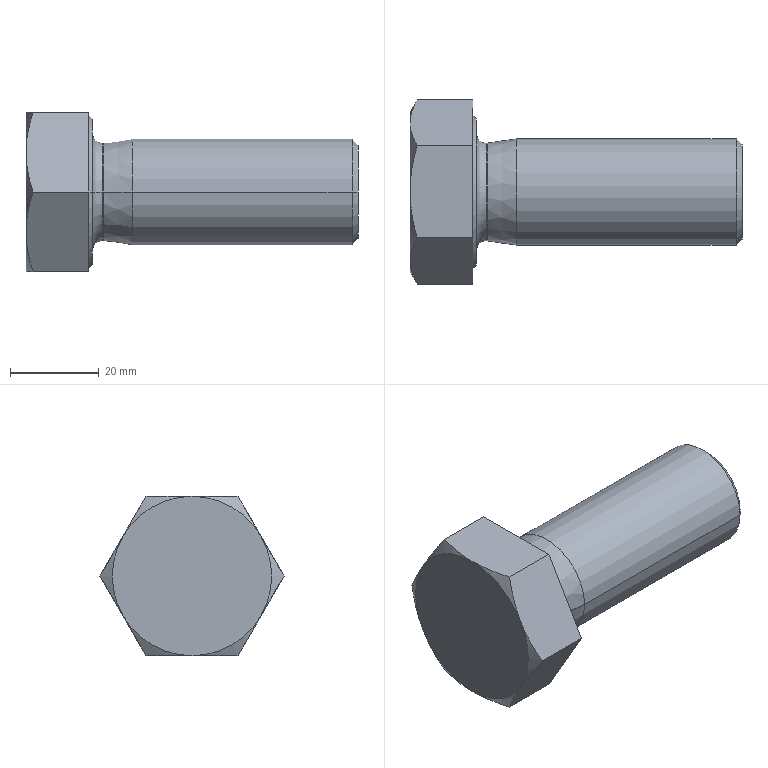Part | SolidWorks | features Chamfer 2, RevCut 2, Revolution 2, Extrusion 1, ICE 1 | 1 solid | 28 faces | box 75 x 41.569 x 36 mm | volume 43357 mm3 | cone 12 | plane 10 | torus 4 | cylinder 2 | commonest cylinder face diameters 24 x2
STEP:
#1=CARTESIAN_POINT('',(15.,-13.226,0.));
#2=VERTEX_POINT('',#1);
#3=CARTESIAN_POINT('',(17.2,-11.026,0.));
#4=VERTEX_POINT('',#3);
#5=CARTESIAN_POINT('',(17.2,-13.226,0.));
#6=DIRECTION('',(0.,0.,-1.));
#7=DIRECTION('',(-1.,0.,0.));
#8=AXIS2_PLACEMENT_3D('',#5,#6,#7);
#9=CIRCLE('',#8,2.2);
#10=EDGE_CURVE('',#2,#4,#9,.T.);
#11=ORIENTED_EDGE('',*,*,#10,.T.);
#12=CARTESIAN_POINT('',(17.2,11.026,0.));
#13=VERTEX_POINT('',#12);
#14=CARTESIAN_POINT('',(17.2,0.,0.));
#15=DIRECTION('',(-1.,0.,0.));
#16=DIRECTION('',(0.,-1.,0.));
#17=AXIS2_PLACEMENT_3D('',#14,#15,#16);
#18=CIRCLE('',#17,11.026);
#19=EDGE_CURVE('',#4,#13,#18,.T.);
#20=ORIENTED_EDGE('',*,*,#19,.T.);
#21=CARTESIAN_POINT('',(15.,13.226,0.));
#22=VERTEX_POINT('',#21);
#23=CARTESIAN_POINT('',(17.2,13.226,0.));
#24=DIRECTION('',(0.,0.,1.));
#25=DIRECTION('',(0.,-1.,0.));
#26=AXIS2_PLACEMENT_3D('',#23,#24,#25);
#27=CIRCLE('',#26,2.2);
#28=EDGE_CURVE('',#22,#13,#27,.T.);
#29=ORIENTED_EDGE('',*,*,#28,.F.);
#30=CARTESIAN_POINT('',(15.,0.,0.));
#31=DIRECTION('',(-1.,0.,0.));
#32=DIRECTION('',(0.,-1.,0.));
#33=AXIS2_PLACEMENT_3D('',#30,#31,#32);
#34=CIRCLE('',#33,13.226);
#35=EDGE_CURVE('',#2,#22,#34,.T.);
#36=ORIENTED_EDGE('',*,*,#35,.F.);
#37=EDGE_LOOP('',(#11,#20,#29,#36));
#38=FACE_OUTER_BOUND('',#37,.T.);
#39=CARTESIAN_POINT('',(17.2,0.,0.));
#40=DIRECTION('',(-1.,0.,0.));
#41=DIRECTION('',(0.,-1.,0.));
#42=AXIS2_PLACEMENT_3D('',#39,#40,#41);
#43=TOROIDAL_SURFACE('',#42,13.226,2.2);
#44=ADVANCED_FACE('',(#38),#43,.F.);
#45=ORIENTED_EDGE('',*,*,#28,.T.);
#46=CARTESIAN_POINT('',(17.2,0.,0.));
#47=DIRECTION('',(-1.,0.,0.));
#48=DIRECTION('',(0.,-1.,0.));
#49=AXIS2_PLACEMENT_3D('',#46,#47,#48);
#50=CIRCLE('',#49,11.026);
#51=EDGE_CURVE('',#13,#4,#50,.T.);
#52=ORIENTED_EDGE('',*,*,#51,.T.);
#53=ORIENTED_EDGE('',*,*,#10,.F.);
#54=CARTESIAN_POINT('',(15.,0.,0.));
#55=DIRECTION('',(-1.,0.,0.));
#56=DIRECTION('',(0.,-1.,0.));
#57=AXIS2_PLACEMENT_3D('',#54,#55,#56);
#58=CIRCLE('',#57,13.226);
#59=EDGE_CURVE('',#22,#2,#58,.T.);
#60=ORIENTED_EDGE('',*,*,#59,.F.);
#61=EDGE_LOOP('',(#45,#52,#53,#60));
#62=FACE_OUTER_BOUND('',#61,.T.);
#63=CARTESIAN_POINT('',(17.2,0.,0.));
#64=DIRECTION('',(-1.,0.,0.));
#65=DIRECTION('',(0.,-1.,0.));
#66=AXIS2_PLACEMENT_3D('',#63,#64,#65);
#67=TOROIDAL_SURFACE('',#66,13.226,2.2);
#68=ADVANCED_FACE('',(#62),#67,.F.);
#69=CARTESIAN_POINT('',(15.,-16.525,0.));
#70=VERTEX_POINT('',#69);
#71=CARTESIAN_POINT('',(15.,16.525,0.));
#72=VERTEX_POINT('',#71);
#73=CARTESIAN_POINT('',(15.,0.,0.));
#74=DIRECTION('',(-1.,0.,0.));
#75=DIRECTION('',(0.,-1.,0.));
#76=AXIS2_PLACEMENT_3D('',#73,#74,#75);
#77=CIRCLE('',#76,16.525);
#78=EDGE_CURVE('',#70,#72,#77,.T.);
#79=ORIENTED_EDGE('',*,*,#78,.T.);
#80=CARTESIAN_POINT('',(14.2,17.325,0.));
#81=VERTEX_POINT('',#80);
#82=CARTESIAN_POINT('',(14.2,17.325,0.));
#83=DIRECTION('',(-0.7071,0.7071,0.));
#84=VECTOR('',#83,1000.);
#85=LINE('',#82,#84);
#86=EDGE_CURVE('',#72,#81,#85,.T.);
#87=ORIENTED_EDGE('',*,*,#86,.T.);
#88=CARTESIAN_POINT('',(14.2,-17.325,0.));
#89=VERTEX_POINT('',#88);
#90=CARTESIAN_POINT('',(14.2,0.,0.));
#91=DIRECTION('',(-1.,0.,0.));
#92=DIRECTION('',(0.,-1.,0.));
#93=AXIS2_PLACEMENT_3D('',#90,#91,#92);
#94=CIRCLE('',#93,17.325);
#95=EDGE_CURVE('',#89,#81,#94,.T.);
#96=ORIENTED_EDGE('',*,*,#95,.F.);
#97=CARTESIAN_POINT('',(14.2,-17.325,0.));
#98=DIRECTION('',(-0.7071,-0.7071,0.));
#99=VECTOR('',#98,1000.);
#100=LINE('',#97,#99);
#101=EDGE_CURVE('',#70,#89,#100,.T.);
#102=ORIENTED_EDGE('',*,*,#101,.F.);
#103=EDGE_LOOP('',(#79,#87,#96,#102));
#104=FACE_OUTER_BOUND('',#103,.T.);
#105=CARTESIAN_POINT('',(14.2,0.,0.));
#106=DIRECTION('',(-1.,0.,0.));
#107=DIRECTION('',(0.,-1.,0.));
#108=AXIS2_PLACEMENT_3D('',#105,#106,#107);
#109=CONICAL_SURFACE('',#108,17.325,0.7854);
#110=ADVANCED_FACE('',(#104),#109,.T.);
#111=CARTESIAN_POINT('',(75.,10.667,0.));
#112=VERTEX_POINT('',#111);
#113=CARTESIAN_POINT('',(75.,-10.667,0.));
#114=VERTEX_POINT('',#113);
#115=CARTESIAN_POINT('',(75.,0.,0.));
#116=DIRECTION('',(1.,0.,0.));
#117=DIRECTION('',(0.,-1.,0.));
#118=AXIS2_PLACEMENT_3D('',#115,#116,#117);
#119=CIRCLE('',#118,10.667);
#120=EDGE_CURVE('',#112,#114,#119,.T.);
#121=ORIENTED_EDGE('',*,*,#120,.F.);
#122=CARTESIAN_POINT('',(73.667,12.,0.));
#123=VERTEX_POINT('',#122);
#124=CARTESIAN_POINT('',(73.667,12.,0.));
#125=DIRECTION('',(-0.7071,0.7071,0.));
#126=VECTOR('',#125,1000.);
#127=LINE('',#124,#126);
#128=EDGE_CURVE('',#112,#123,#127,.T.);
#129=ORIENTED_EDGE('',*,*,#128,.T.);
#130=CARTESIAN_POINT('',(73.667,-12.,0.));
#131=VERTEX_POINT('',#130);
#132=CARTESIAN_POINT('',(73.667,0.,0.));
#133=DIRECTION('',(-1.,0.,0.));
#134=DIRECTION('',(0.,-1.,0.));
#135=AXIS2_PLACEMENT_3D('',#132,#133,#134);
#136=CIRCLE('',#135,12.);
#137=EDGE_CURVE('',#131,#123,#136,.T.);
#138=ORIENTED_EDGE('',*,*,#137,.F.);
#139=CARTESIAN_POINT('',(73.667,-12.,0.));
#140=DIRECTION('',(-0.7071,-0.7071,0.));
#141=VECTOR('',#140,1000.);
#142=LINE('',#139,#141);
#143=EDGE_CURVE('',#114,#131,#142,.T.);
#144=ORIENTED_EDGE('',*,*,#143,.F.);
#145=EDGE_LOOP('',(#121,#129,#138,#144));
#146=FACE_OUTER_BOUND('',#145,.T.);
#147=CARTESIAN_POINT('',(73.667,0.,0.));
#148=DIRECTION('',(-1.,0.,0.));
#149=DIRECTION('',(0.,-1.,0.));
#150=AXIS2_PLACEMENT_3D('',#147,#148,#149);
#151=CONICAL_SURFACE('',#150,12.,0.7854);
#152=ADVANCED_FACE('',(#146),#151,.T.);
#153=ORIENTED_EDGE('',*,*,#51,.F.);
#154=CARTESIAN_POINT('',(17.519,11.049,0.));
#155=VERTEX_POINT('',#154);
#156=CARTESIAN_POINT('',(17.2,13.226,0.));
#157=DIRECTION('',(0.,0.,1.));
#158=DIRECTION('',(0.,-1.,0.));
#159=AXIS2_PLACEMENT_3D('',#156,#157,#158);
#160=CIRCLE('',#159,2.2);
#161=EDGE_CURVE('',#13,#155,#160,.T.);
#162=ORIENTED_EDGE('',*,*,#161,.T.);
#163=CARTESIAN_POINT('',(17.519,-11.049,0.));
#164=VERTEX_POINT('',#163);
#165=CARTESIAN_POINT('',(17.519,0.,0.));
#166=DIRECTION('',(-1.,0.,0.));
#167=DIRECTION('',(0.,-1.,0.));
#168=AXIS2_PLACEMENT_3D('',#165,#166,#167);
#169=CIRCLE('',#168,11.049);
#170=EDGE_CURVE('',#155,#164,#169,.T.);
#171=ORIENTED_EDGE('',*,*,#170,.T.);
#172=CARTESIAN_POINT('',(17.2,-13.226,0.));
#173=DIRECTION('',(0.,0.,-1.));
#174=DIRECTION('',(-1.,0.,0.));
#175=AXIS2_PLACEMENT_3D('',#172,#173,#174);
#176=CIRCLE('',#175,2.2);
#177=EDGE_CURVE('',#4,#164,#176,.T.);
#178=ORIENTED_EDGE('',*,*,#177,.F.);
#179=EDGE_LOOP('',(#153,#162,#171,#178));
#180=FACE_OUTER_BOUND('',#179,.T.);
#181=CARTESIAN_POINT('',(17.2,0.,0.));
#182=DIRECTION('',(-1.,0.,0.));
#183=DIRECTION('',(0.,-1.,0.));
#184=AXIS2_PLACEMENT_3D('',#181,#182,#183);
#185=TOROIDAL_SURFACE('',#184,13.226,2.2);
#186=ADVANCED_FACE('',(#180),#185,.F.);
#187=ORIENTED_EDGE('',*,*,#137,.T.);
#188=CARTESIAN_POINT('',(24.,12.,0.));
#189=VERTEX_POINT('',#188);
#190=CARTESIAN_POINT('',(15.,12.,0.));
#191=DIRECTION('',(-1.,0.,0.));
#192=VECTOR('',#191,1000.);
#193=LINE('',#190,#192);
#194=EDGE_CURVE('',#123,#189,#193,.T.);
#195=ORIENTED_EDGE('',*,*,#194,.T.);
#196=CARTESIAN_POINT('',(24.,-12.,0.));
#197=VERTEX_POINT('',#196);
#198=CARTESIAN_POINT('',(24.,0.,0.));
#199=DIRECTION('',(-1.,0.,0.));
#200=DIRECTION('',(0.,-1.,0.));
#201=AXIS2_PLACEMENT_3D('',#198,#199,#200);
#202=CIRCLE('',#201,12.);
#203=EDGE_CURVE('',#197,#189,#202,.T.);
#204=ORIENTED_EDGE('',*,*,#203,.F.);
#205=CARTESIAN_POINT('',(15.,-12.,0.));
#206=DIRECTION('',(-1.,0.,0.));
#207=VECTOR('',#206,1000.);
#208=LINE('',#205,#207);
#209=EDGE_CURVE('',#131,#197,#208,.T.);
#210=ORIENTED_EDGE('',*,*,#209,.F.);
#211=EDGE_LOOP('',(#187,#195,#204,#210));
#212=FACE_OUTER_BOUND('',#211,.T.);
#213=CARTESIAN_POINT('',(15.,0.,0.));
#214=DIRECTION('',(-1.,0.,0.));
#215=DIRECTION('',(0.,-1.,0.));
#216=AXIS2_PLACEMENT_3D('',#213,#214,#215);
#217=CYLINDRICAL_SURFACE('',#216,12.);
#218=ADVANCED_FACE('',(#212),#217,.T.);
#219=CARTESIAN_POINT('',(17.519,0.,0.));
#220=DIRECTION('',(-1.,0.,0.));
#221=DIRECTION('',(0.,-1.,0.));
#222=AXIS2_PLACEMENT_3D('',#219,#220,#221);
#223=CIRCLE('',#222,11.049);
#224=EDGE_CURVE('',#164,#155,#223,.T.);
#225=ORIENTED_EDGE('',*,*,#224,.F.);
#226=CARTESIAN_POINT('',(24.,-12.,0.));
#227=DIRECTION('',(0.9894,-0.1452,0.));
#228=VECTOR('',#227,1000.);
#229=LINE('',#226,#228);
#230=EDGE_CURVE('',#164,#197,#229,.T.);
#231=ORIENTED_EDGE('',*,*,#230,.T.);
#232=ORIENTED_EDGE('',*,*,#203,.T.);
#233=CARTESIAN_POINT('',(24.,12.,0.));
#234=DIRECTION('',(0.9894,0.1452,0.));
#235=VECTOR('',#234,1000.);
#236=LINE('',#233,#235);
#237=EDGE_CURVE('',#155,#189,#236,.T.);
#238=ORIENTED_EDGE('',*,*,#237,.F.);
#239=EDGE_LOOP('',(#225,#231,#232,#238));
#240=FACE_OUTER_BOUND('',#239,.T.);
#241=CARTESIAN_POINT('',(24.,0.,0.));
#242=DIRECTION('',(1.,0.,0.));
#243=DIRECTION('',(0.,1.,0.));
#244=AXIS2_PLACEMENT_3D('',#241,#242,#243);
#245=CONICAL_SURFACE('',#244,12.,0.1457);
#246=ADVANCED_FACE('',(#240),#245,.T.);
#247=ORIENTED_EDGE('',*,*,#35,.T.);
#248=ORIENTED_EDGE('',*,*,#59,.T.);
#249=EDGE_LOOP('',(#247,#248));
#250=FACE_BOUND('',#249,.T.);
#251=ORIENTED_EDGE('',*,*,#78,.F.);
#252=CARTESIAN_POINT('',(15.,0.,0.));
#253=DIRECTION('',(-1.,0.,0.));
#254=DIRECTION('',(0.,-1.,0.));
#255=AXIS2_PLACEMENT_3D('',#252,#253,#254);
#256=CIRCLE('',#255,16.525);
#257=EDGE_CURVE('',#72,#70,#256,.T.);
#258=ORIENTED_EDGE('',*,*,#257,.F.);
#259=EDGE_LOOP('',(#251,#258));
#260=FACE_OUTER_BOUND('',#259,.T.);
#261=CARTESIAN_POINT('',(15.,10.392,-18.));
#262=DIRECTION('',(1.,0.,0.));
#263=DIRECTION('',(0.,0.,-1.));
#264=AXIS2_PLACEMENT_3D('',#261,#262,#263);
#265=PLANE('',#264);
#266=ADVANCED_FACE('',(#250,#260),#265,.T.);
#267=ORIENTED_EDGE('',*,*,#230,.F.);
#268=ORIENTED_EDGE('',*,*,#170,.F.);
#269=ORIENTED_EDGE('',*,*,#237,.T.);
#270=CARTESIAN_POINT('',(24.,0.,0.));
#271=DIRECTION('',(-1.,0.,0.));
#272=DIRECTION('',(0.,-1.,0.));
#273=AXIS2_PLACEMENT_3D('',#270,#271,#272);
#274=CIRCLE('',#273,12.);
#275=EDGE_CURVE('',#189,#197,#274,.T.);
#276=ORIENTED_EDGE('',*,*,#275,.T.);
#277=EDGE_LOOP('',(#267,#268,#269,#276));
#278=FACE_OUTER_BOUND('',#277,.T.);
#279=CARTESIAN_POINT('',(24.,0.,0.));
#280=DIRECTION('',(1.,0.,0.));
#281=DIRECTION('',(0.,1.,0.));
#282=AXIS2_PLACEMENT_3D('',#279,#280,#281);
#283=CONICAL_SURFACE('',#282,12.,0.1457);
#284=ADVANCED_FACE('',(#278),#283,.T.);
#285=ORIENTED_EDGE('',*,*,#194,.F.);
#286=CARTESIAN_POINT('',(73.667,0.,0.));
#287=DIRECTION('',(-1.,0.,0.));
#288=DIRECTION('',(0.,-1.,0.));
#289=AXIS2_PLACEMENT_3D('',#286,#287,#288);
#290=CIRCLE('',#289,12.);
#291=EDGE_CURVE('',#123,#131,#290,.T.);
#292=ORIENTED_EDGE('',*,*,#291,.T.);
#293=ORIENTED_EDGE('',*,*,#209,.T.);
#294=ORIENTED_EDGE('',*,*,#275,.F.);
#295=EDGE_LOOP('',(#285,#292,#293,#294));
#296=FACE_OUTER_BOUND('',#295,.T.);
#297=CARTESIAN_POINT('',(15.,0.,0.));
#298=DIRECTION('',(-1.,0.,0.));
#299=DIRECTION('',(0.,-1.,0.));
#300=AXIS2_PLACEMENT_3D('',#297,#298,#299);
#301=CYLINDRICAL_SURFACE('',#300,12.);
#302=ADVANCED_FACE('',(#296),#301,.T.);
#303=CARTESIAN_POINT('',(75.,0.,0.));
#304=DIRECTION('',(1.,0.,0.));
#305=DIRECTION('',(0.,-1.,0.));
#306=AXIS2_PLACEMENT_3D('',#303,#304,#305);
#307=CIRCLE('',#306,10.667);
#308=EDGE_CURVE('',#114,#112,#307,.T.);
#309=ORIENTED_EDGE('',*,*,#308,.T.);
#310=ORIENTED_EDGE('',*,*,#120,.T.);
#311=EDGE_LOOP('',(#309,#310));
#312=FACE_OUTER_BOUND('',#311,.T.);
#313=CARTESIAN_POINT('',(75.,12.,0.));
#314=DIRECTION('',(-1.,0.,0.));
#315=DIRECTION('',(0.,-1.,0.));
#316=AXIS2_PLACEMENT_3D('',#313,#314,#315);
#317=PLANE('',#316);
#318=ADVANCED_FACE('',(#312),#317,.F.);
#319=ORIENTED_EDGE('',*,*,#19,.F.);
#320=ORIENTED_EDGE('',*,*,#177,.T.);
#321=ORIENTED_EDGE('',*,*,#224,.T.);
#322=ORIENTED_EDGE('',*,*,#161,.F.);
#323=EDGE_LOOP('',(#319,#320,#321,#322));
#324=FACE_OUTER_BOUND('',#323,.T.);
#325=CARTESIAN_POINT('',(17.2,0.,0.));
#326=DIRECTION('',(-1.,0.,0.));
#327=DIRECTION('',(0.,-1.,0.));
#328=AXIS2_PLACEMENT_3D('',#325,#326,#327);
#329=TOROIDAL_SURFACE('',#328,13.226,2.2);
#330=ADVANCED_FACE('',(#324),#329,.F.);
#331=ORIENTED_EDGE('',*,*,#128,.F.);
#332=ORIENTED_EDGE('',*,*,#308,.F.);
#333=ORIENTED_EDGE('',*,*,#143,.T.);
#334=ORIENTED_EDGE('',*,*,#291,.F.);
#335=EDGE_LOOP('',(#331,#332,#333,#334));
#336=FACE_OUTER_BOUND('',#335,.T.);
#337=CARTESIAN_POINT('',(73.667,0.,0.));
#338=DIRECTION('',(-1.,0.,0.));
#339=DIRECTION('',(0.,-1.,0.));
#340=AXIS2_PLACEMENT_3D('',#337,#338,#339);
#341=CONICAL_SURFACE('',#340,12.,0.7854);
#342=ADVANCED_FACE('',(#336),#341,.T.);
#343=ORIENTED_EDGE('',*,*,#95,.T.);
#344=CARTESIAN_POINT('',(14.2,0.,0.));
#345=DIRECTION('',(-1.,0.,0.));
#346=DIRECTION('',(0.,-1.,0.));
#347=AXIS2_PLACEMENT_3D('',#344,#345,#346);
#348=CIRCLE('',#347,17.325);
#349=EDGE_CURVE('',#81,#89,#348,.T.);
#350=ORIENTED_EDGE('',*,*,#349,.T.);
#351=EDGE_LOOP('',(#343,#350));
#352=FACE_BOUND('',#351,.T.);
#353=CARTESIAN_POINT('',(14.2,-10.392,-18.));
#354=VERTEX_POINT('',#353);
#355=CARTESIAN_POINT('',(14.2,10.392,-18.));
#356=VERTEX_POINT('',#355);
#357=CARTESIAN_POINT('',(14.2,-10.392,-18.));
#358=DIRECTION('',(0.,1.,0.));
#359=VECTOR('',#358,1000.);
#360=LINE('',#357,#359);
#361=EDGE_CURVE('',#354,#356,#360,.T.);
#362=ORIENTED_EDGE('',*,*,#361,.T.);
#363=CARTESIAN_POINT('',(14.2,20.785,0.));
#364=VERTEX_POINT('',#363);
#365=CARTESIAN_POINT('',(14.2,10.392,-18.));
#366=DIRECTION('',(0.,0.5,0.866));
#367=VECTOR('',#366,1000.);
#368=LINE('',#365,#367);
#369=EDGE_CURVE('',#356,#364,#368,.T.);
#370=ORIENTED_EDGE('',*,*,#369,.T.);
#371=CARTESIAN_POINT('',(14.2,10.392,18.));
#372=VERTEX_POINT('',#371);
#373=CARTESIAN_POINT('',(14.2,20.785,0.));
#374=DIRECTION('',(0.,-0.5,0.866));
#375=VECTOR('',#374,1000.);
#376=LINE('',#373,#375);
#377=EDGE_CURVE('',#364,#372,#376,.T.);
#378=ORIENTED_EDGE('',*,*,#377,.T.);
#379=CARTESIAN_POINT('',(14.2,-10.392,18.));
#380=VERTEX_POINT('',#379);
#381=CARTESIAN_POINT('',(14.2,10.392,18.));
#382=DIRECTION('',(0.,-1.,0.));
#383=VECTOR('',#382,1000.);
#384=LINE('',#381,#383);
#385=EDGE_CURVE('',#372,#380,#384,.T.);
#386=ORIENTED_EDGE('',*,*,#385,.T.);
#387=CARTESIAN_POINT('',(14.2,-20.785,0.));
#388=VERTEX_POINT('',#387);
#389=CARTESIAN_POINT('',(14.2,-10.392,18.));
#390=DIRECTION('',(0.,-0.5,-0.866));
#391=VECTOR('',#390,1000.);
#392=LINE('',#389,#391);
#393=EDGE_CURVE('',#380,#388,#392,.T.);
#394=ORIENTED_EDGE('',*,*,#393,.T.);
#395=CARTESIAN_POINT('',(14.2,-20.785,0.));
#396=DIRECTION('',(0.,0.5,-0.866));
#397=VECTOR('',#396,1000.);
#398=LINE('',#395,#397);
#399=EDGE_CURVE('',#388,#354,#398,.T.);
#400=ORIENTED_EDGE('',*,*,#399,.T.);
#401=EDGE_LOOP('',(#362,#370,#378,#386,#394,#400));
#402=FACE_OUTER_BOUND('',#401,.T.);
#403=CARTESIAN_POINT('',(14.2,-17.325,0.));
#404=DIRECTION('',(1.,0.,0.));
#405=DIRECTION('',(0.,1.,0.));
#406=AXIS2_PLACEMENT_3D('',#403,#404,#405);
#407=PLANE('',#406);
#408=ADVANCED_FACE('',(#352,#402),#407,.T.);
#409=ORIENTED_EDGE('',*,*,#86,.F.);
#410=ORIENTED_EDGE('',*,*,#257,.T.);
#411=ORIENTED_EDGE('',*,*,#101,.T.);
#412=ORIENTED_EDGE('',*,*,#349,.F.);
#413=EDGE_LOOP('',(#409,#410,#411,#412));
#414=FACE_OUTER_BOUND('',#413,.T.);
#415=CARTESIAN_POINT('',(14.2,0.,0.));
#416=DIRECTION('',(-1.,0.,0.));
#417=DIRECTION('',(0.,-1.,0.));
#418=AXIS2_PLACEMENT_3D('',#415,#416,#417);
#419=CONICAL_SURFACE('',#418,17.325,0.7854);
#420=ADVANCED_FACE('',(#414),#419,.T.);
#421=CARTESIAN_POINT('',(0.,0.,-18.));
#422=VERTEX_POINT('',#421);
#423=CARTESIAN_POINT('',(0.,15.588,-9.));
#424=VERTEX_POINT('',#423);
#425=CARTESIAN_POINT('',(0.,0.,0.));
#426=DIRECTION('',(1.,0.,0.));
#427=DIRECTION('',(0.,0.,-1.));
#428=AXIS2_PLACEMENT_3D('',#425,#426,#427);
#429=CIRCLE('',#428,18.);
#430=EDGE_CURVE('',#422,#424,#429,.T.);
#431=ORIENTED_EDGE('',*,*,#430,.F.);
#432=CARTESIAN_POINT('',(0.,-15.588,-9.));
#433=VERTEX_POINT('',#432);
#434=CARTESIAN_POINT('',(0.,0.,0.));
#435=DIRECTION('',(1.,0.,0.));
#436=DIRECTION('',(0.,0.,-1.));
#437=AXIS2_PLACEMENT_3D('',#434,#435,#436);
#438=CIRCLE('',#437,18.);
#439=EDGE_CURVE('',#433,#422,#438,.T.);
#440=ORIENTED_EDGE('',*,*,#439,.F.);
#441=CARTESIAN_POINT('',(0.,-15.588,9.));
#442=VERTEX_POINT('',#441);
#443=CARTESIAN_POINT('',(0.,0.,0.));
#444=DIRECTION('',(1.,0.,0.));
#445=DIRECTION('',(0.,0.,-1.));
#446=AXIS2_PLACEMENT_3D('',#443,#444,#445);
#447=CIRCLE('',#446,18.);
#448=EDGE_CURVE('',#442,#433,#447,.T.);
#449=ORIENTED_EDGE('',*,*,#448,.F.);
#450=CARTESIAN_POINT('',(0.,0.,18.));
#451=VERTEX_POINT('',#450);
#452=CARTESIAN_POINT('',(0.,0.,0.));
#453=DIRECTION('',(1.,0.,0.));
#454=DIRECTION('',(0.,0.,-1.));
#455=AXIS2_PLACEMENT_3D('',#452,#453,#454);
#456=CIRCLE('',#455,18.);
#457=EDGE_CURVE('',#451,#442,#456,.T.);
#458=ORIENTED_EDGE('',*,*,#457,.F.);
#459=CARTESIAN_POINT('',(0.,15.588,9.));
#460=VERTEX_POINT('',#459);
#461=CARTESIAN_POINT('',(0.,0.,0.));
#462=DIRECTION('',(-1.,0.,0.));
#463=DIRECTION('',(0.,0.,1.));
#464=AXIS2_PLACEMENT_3D('',#461,#462,#463);
#465=CIRCLE('',#464,18.);
#466=EDGE_CURVE('',#451,#460,#465,.T.);
#467=ORIENTED_EDGE('',*,*,#466,.T.);
#468=CARTESIAN_POINT('',(0.,0.,0.));
#469=DIRECTION('',(1.,0.,0.));
#470=DIRECTION('',(0.,0.,-1.));
#471=AXIS2_PLACEMENT_3D('',#468,#469,#470);
#472=CIRCLE('',#471,18.);
#473=EDGE_CURVE('',#424,#460,#472,.T.);
#474=ORIENTED_EDGE('',*,*,#473,.F.);
#475=EDGE_LOOP('',(#431,#440,#449,#458,#467,#474));
#476=FACE_OUTER_BOUND('',#475,.T.);
#477=CARTESIAN_POINT('',(0.,10.392,-18.));
#478=DIRECTION('',(1.,0.,0.));
#479=DIRECTION('',(0.,0.,-1.));
#480=AXIS2_PLACEMENT_3D('',#477,#478,#479);
#481=PLANE('',#480);
#482=ADVANCED_FACE('',(#476),#481,.F.);
#483=CARTESIAN_POINT('',(1.608,10.392,-18.));
#484=VERTEX_POINT('',#483);
#485=CARTESIAN_POINT('',(0.,15.588,-9.));
#486=CARTESIAN_POINT('',(0.,15.368,-9.382));
#487=CARTESIAN_POINT('',(0.009429,15.146,-9.766));
#488=CARTESIAN_POINT('',(0.04683,14.705,-10.53));
#489=CARTESIAN_POINT('',(0.07476,14.485,-10.91));
#490=CARTESIAN_POINT('',(0.1851,13.828,-12.049));
#491=CARTESIAN_POINT('',(0.294,13.393,-12.803));
#492=CARTESIAN_POINT('',(0.714,12.095,-15.051));
#493=CARTESIAN_POINT('',(1.118,11.24,-16.531));
#494=CARTESIAN_POINT('',(1.608,10.392,-18.));
#495=B_SPLINE_CURVE_WITH_KNOTS('',3,(#485,#486,#487,#488,#489,#490,#491,#492,#493,#494),.UNSPECIFIED.,.F.,.F.,(4,2,2,2,4),(0.01052,0.01183,0.01313,0.01575,0.02099),.UNSPECIFIED.);
#496=EDGE_CURVE('',#424,#484,#495,.T.);
#497=ORIENTED_EDGE('',*,*,#496,.T.);
#498=CARTESIAN_POINT('',(1.608,10.392,-18.));
#499=CARTESIAN_POINT('',(1.123,8.712,-18.));
#500=CARTESIAN_POINT('',(0.7186,7.01,-18.));
#501=CARTESIAN_POINT('',(0.296,4.406,-18.));
#502=CARTESIAN_POINT('',(0.1858,3.529,-18.));
#503=CARTESIAN_POINT('',(0.03734,1.76,-18.));
#504=CARTESIAN_POINT('',(0.,0.8787,-18.));
#505=CARTESIAN_POINT('',(0.,0.,-18.));
#506=B_SPLINE_CURVE_WITH_KNOTS('',3,(#498,#499,#500,#501,#502,#503,#504,#505),.UNSPECIFIED.,.F.,.F.,(4,2,2,4),(0.007574,0.01282,0.01544,0.01807),.UNSPECIFIED.);
#507=EDGE_CURVE('',#484,#422,#506,.T.);
#508=ORIENTED_EDGE('',*,*,#507,.T.);
#509=ORIENTED_EDGE('',*,*,#430,.T.);
#510=EDGE_LOOP('',(#497,#508,#509));
#511=FACE_OUTER_BOUND('',#510,.T.);
#512=CARTESIAN_POINT('',(0.,0.,0.));
#513=DIRECTION('',(1.,0.,0.));
#514=DIRECTION('',(0.,0.,1.));
#515=AXIS2_PLACEMENT_3D('',#512,#513,#514);
#516=CONICAL_SURFACE('',#515,18.,1.047);
#517=ADVANCED_FACE('',(#511),#516,.T.);
#518=CARTESIAN_POINT('',(1.608,20.785,0.));
#519=VERTEX_POINT('',#518);
#520=CARTESIAN_POINT('',(0.,15.588,9.));
#521=CARTESIAN_POINT('',(0.,15.809,8.618));
#522=CARTESIAN_POINT('',(0.009429,16.031,8.234));
#523=CARTESIAN_POINT('',(0.04683,16.472,7.47));
#524=CARTESIAN_POINT('',(0.07476,16.691,7.09));
#525=CARTESIAN_POINT('',(0.1851,17.349,5.951));
#526=CARTESIAN_POINT('',(0.294,17.784,5.197));
#527=CARTESIAN_POINT('',(0.714,19.082,2.949));
#528=CARTESIAN_POINT('',(1.118,19.937,1.469));
#529=CARTESIAN_POINT('',(1.608,20.785,0.));
#530=B_SPLINE_CURVE_WITH_KNOTS('',3,(#520,#521,#522,#523,#524,#525,#526,#527,#528,#529),.UNSPECIFIED.,.F.,.F.,(4,2,2,2,4),(0.01052,0.01183,0.01313,0.01575,0.02099),.UNSPECIFIED.);
#531=EDGE_CURVE('',#460,#519,#530,.T.);
#532=ORIENTED_EDGE('',*,*,#531,.T.);
#533=CARTESIAN_POINT('',(1.608,20.785,0.));
#534=CARTESIAN_POINT('',(1.117,19.935,-1.472));
#535=CARTESIAN_POINT('',(0.7126,19.078,-2.955));
#536=CARTESIAN_POINT('',(0.1532,17.348,-5.952));
#537=CARTESIAN_POINT('',(0.,16.474,-7.467));
#538=CARTESIAN_POINT('',(0.,15.588,-9.));
#539=B_SPLINE_CURVE_WITH_KNOTS('',3,(#533,#534,#535,#536,#537,#538),.UNSPECIFIED.,.F.,.F.,(4,2,4),(0.000000238,0.005258,0.01052),.UNSPECIFIED.);
#540=EDGE_CURVE('',#519,#424,#539,.T.);
#541=ORIENTED_EDGE('',*,*,#540,.T.);
#542=ORIENTED_EDGE('',*,*,#473,.T.);
#543=EDGE_LOOP('',(#532,#541,#542));
#544=FACE_OUTER_BOUND('',#543,.T.);
#545=CARTESIAN_POINT('',(0.,0.,0.));
#546=DIRECTION('',(1.,0.,0.));
#547=DIRECTION('',(0.,0.,1.));
#548=AXIS2_PLACEMENT_3D('',#545,#546,#547);
#549=CONICAL_SURFACE('',#548,18.,1.047);
#550=ADVANCED_FACE('',(#544),#549,.T.);
#551=CARTESIAN_POINT('',(1.608,10.392,18.));
#552=VERTEX_POINT('',#551);
#553=CARTESIAN_POINT('',(1.608,10.392,18.));
#554=CARTESIAN_POINT('',(1.117,11.242,16.528));
#555=CARTESIAN_POINT('',(0.7126,12.099,15.045));
#556=CARTESIAN_POINT('',(0.1532,13.829,12.048));
#557=CARTESIAN_POINT('',(0.,14.703,10.533));
#558=CARTESIAN_POINT('',(0.,15.588,9.));
#559=B_SPLINE_CURVE_WITH_KNOTS('',3,(#553,#554,#555,#556,#557,#558),.UNSPECIFIED.,.F.,.F.,(4,2,4),(0.000000238,0.005258,0.01052),.UNSPECIFIED.);
#560=EDGE_CURVE('',#552,#460,#559,.T.);
#561=ORIENTED_EDGE('',*,*,#560,.T.);
#562=ORIENTED_EDGE('',*,*,#466,.F.);
#563=CARTESIAN_POINT('',(0.,0.,18.));
#564=CARTESIAN_POINT('',(0.,0.8787,18.));
#565=CARTESIAN_POINT('',(0.03734,1.76,18.));
#566=CARTESIAN_POINT('',(0.1858,3.529,18.));
#567=CARTESIAN_POINT('',(0.296,4.406,18.));
#568=CARTESIAN_POINT('',(0.7186,7.01,18.));
#569=CARTESIAN_POINT('',(1.123,8.712,18.));
#570=CARTESIAN_POINT('',(1.608,10.392,18.));
#571=B_SPLINE_CURVE_WITH_KNOTS('',3,(#563,#564,#565,#566,#567,#568,#569,#570),.UNSPECIFIED.,.F.,.F.,(4,2,2,4),(0.0291,0.03173,0.03436,0.03962),.UNSPECIFIED.);
#572=EDGE_CURVE('',#451,#552,#571,.T.);
#573=ORIENTED_EDGE('',*,*,#572,.T.);
#574=EDGE_LOOP('',(#561,#562,#573));
#575=FACE_OUTER_BOUND('',#574,.T.);
#576=CARTESIAN_POINT('',(0.,0.,0.));
#577=DIRECTION('',(1.,0.,0.));
#578=DIRECTION('',(0.,0.,1.));
#579=AXIS2_PLACEMENT_3D('',#576,#577,#578);
#580=CONICAL_SURFACE('',#579,18.,1.047);
#581=ADVANCED_FACE('',(#575),#580,.T.);
#582=CARTESIAN_POINT('',(1.608,-10.392,18.));
#583=VERTEX_POINT('',#582);
#584=CARTESIAN_POINT('',(1.608,-10.392,18.));
#585=CARTESIAN_POINT('',(1.364,-9.547,18.));
#586=CARTESIAN_POINT('',(1.14,-8.694,18.));
#587=CARTESIAN_POINT('',(0.7423,-6.969,18.));
#588=CARTESIAN_POINT('',(0.5706,-6.103,18.));
#589=CARTESIAN_POINT('',(0.151,-3.501,18.));
#590=CARTESIAN_POINT('',(0.,-1.756,18.));
#591=CARTESIAN_POINT('',(0.,0.,18.));
#592=B_SPLINE_CURVE_WITH_KNOTS('',3,(#584,#585,#586,#587,#588,#589,#590,#591),.UNSPECIFIED.,.F.,.F.,(4,2,2,4),(0.01858,0.02121,0.02384,0.0291),.UNSPECIFIED.);
#593=EDGE_CURVE('',#583,#451,#592,.T.);
#594=ORIENTED_EDGE('',*,*,#593,.T.);
#595=ORIENTED_EDGE('',*,*,#457,.T.);
#596=CARTESIAN_POINT('',(0.,-15.588,9.));
#597=CARTESIAN_POINT('',(0.,-15.368,9.382));
#598=CARTESIAN_POINT('',(0.009429,-15.146,9.766));
#599=CARTESIAN_POINT('',(0.04683,-14.705,10.53));
#600=CARTESIAN_POINT('',(0.07476,-14.485,10.91));
#601=CARTESIAN_POINT('',(0.1851,-13.828,12.049));
#602=CARTESIAN_POINT('',(0.294,-13.393,12.803));
#603=CARTESIAN_POINT('',(0.714,-12.095,15.051));
#604=CARTESIAN_POINT('',(1.118,-11.24,16.531));
#605=CARTESIAN_POINT('',(1.608,-10.392,18.));
#606=B_SPLINE_CURVE_WITH_KNOTS('',3,(#596,#597,#598,#599,#600,#601,#602,#603,#604,#605),.UNSPECIFIED.,.F.,.F.,(4,2,2,2,4),(0.01052,0.01183,0.01313,0.01575,0.02099),.UNSPECIFIED.);
#607=EDGE_CURVE('',#442,#583,#606,.T.);
#608=ORIENTED_EDGE('',*,*,#607,.T.);
#609=EDGE_LOOP('',(#594,#595,#608));
#610=FACE_OUTER_BOUND('',#609,.T.);
#611=CARTESIAN_POINT('',(0.,0.,0.));
#612=DIRECTION('',(1.,0.,0.));
#613=DIRECTION('',(0.,0.,1.));
#614=AXIS2_PLACEMENT_3D('',#611,#612,#613);
#615=CONICAL_SURFACE('',#614,18.,1.047);
#616=ADVANCED_FACE('',(#610),#615,.T.);
#617=CARTESIAN_POINT('',(1.608,-10.392,-18.));
#618=VERTEX_POINT('',#617);
#619=CARTESIAN_POINT('',(0.,0.,-18.));
#620=CARTESIAN_POINT('',(0.,-1.756,-18.));
#621=CARTESIAN_POINT('',(0.151,-3.501,-18.));
#622=CARTESIAN_POINT('',(0.5706,-6.103,-18.));
#623=CARTESIAN_POINT('',(0.7423,-6.969,-18.));
#624=CARTESIAN_POINT('',(1.14,-8.694,-18.));
#625=CARTESIAN_POINT('',(1.364,-9.547,-18.));
#626=CARTESIAN_POINT('',(1.608,-10.392,-18.));
#627=B_SPLINE_CURVE_WITH_KNOTS('',3,(#619,#620,#621,#622,#623,#624,#625,#626),.UNSPECIFIED.,.F.,.F.,(4,2,2,4),(0.01807,0.02331,0.02593,0.02855),.UNSPECIFIED.);
#628=EDGE_CURVE('',#422,#618,#627,.T.);
#629=ORIENTED_EDGE('',*,*,#628,.T.);
#630=CARTESIAN_POINT('',(1.608,-10.392,-18.));
#631=CARTESIAN_POINT('',(1.117,-11.242,-16.528));
#632=CARTESIAN_POINT('',(0.7126,-12.099,-15.045));
#633=CARTESIAN_POINT('',(0.1532,-13.829,-12.048));
#634=CARTESIAN_POINT('',(0.,-14.703,-10.533));
#635=CARTESIAN_POINT('',(0.,-15.588,-9.));
#636=B_SPLINE_CURVE_WITH_KNOTS('',3,(#630,#631,#632,#633,#634,#635),.UNSPECIFIED.,.F.,.F.,(4,2,4),(0.000000238,0.005258,0.01052),.UNSPECIFIED.);
#637=EDGE_CURVE('',#618,#433,#636,.T.);
#638=ORIENTED_EDGE('',*,*,#637,.T.);
#639=ORIENTED_EDGE('',*,*,#439,.T.);
#640=EDGE_LOOP('',(#629,#638,#639));
#641=FACE_OUTER_BOUND('',#640,.T.);
#642=CARTESIAN_POINT('',(0.,0.,0.));
#643=DIRECTION('',(1.,0.,0.));
#644=DIRECTION('',(0.,0.,1.));
#645=AXIS2_PLACEMENT_3D('',#642,#643,#644);
#646=CONICAL_SURFACE('',#645,18.,1.047);
#647=ADVANCED_FACE('',(#641),#646,.T.);
#648=CARTESIAN_POINT('',(1.608,-20.785,0.));
#649=VERTEX_POINT('',#648);
#650=CARTESIAN_POINT('',(1.608,-20.785,0.));
#651=CARTESIAN_POINT('',(1.117,-19.935,1.472));
#652=CARTESIAN_POINT('',(0.7126,-19.078,2.955));
#653=CARTESIAN_POINT('',(0.1532,-17.348,5.952));
#654=CARTESIAN_POINT('',(0.,-16.474,7.467));
#655=CARTESIAN_POINT('',(0.,-15.588,9.));
#656=B_SPLINE_CURVE_WITH_KNOTS('',3,(#650,#651,#652,#653,#654,#655),.UNSPECIFIED.,.F.,.F.,(4,2,4),(0.000000238,0.005258,0.01052),.UNSPECIFIED.);
#657=EDGE_CURVE('',#649,#442,#656,.T.);
#658=ORIENTED_EDGE('',*,*,#657,.T.);
#659=ORIENTED_EDGE('',*,*,#448,.T.);
#660=CARTESIAN_POINT('',(0.,-15.588,-9.));
#661=CARTESIAN_POINT('',(0.,-15.809,-8.618));
#662=CARTESIAN_POINT('',(0.009429,-16.031,-8.234));
#663=CARTESIAN_POINT('',(0.04683,-16.472,-7.47));
#664=CARTESIAN_POINT('',(0.07476,-16.691,-7.09));
#665=CARTESIAN_POINT('',(0.1851,-17.349,-5.951));
#666=CARTESIAN_POINT('',(0.294,-17.784,-5.197));
#667=CARTESIAN_POINT('',(0.714,-19.082,-2.949));
#668=CARTESIAN_POINT('',(1.118,-19.937,-1.469));
#669=CARTESIAN_POINT('',(1.608,-20.785,0.));
#670=B_SPLINE_CURVE_WITH_KNOTS('',3,(#660,#661,#662,#663,#664,#665,#666,#667,#668,#669),.UNSPECIFIED.,.F.,.F.,(4,2,2,2,4),(0.01052,0.01183,0.01313,0.01575,0.02099),.UNSPECIFIED.);
#671=EDGE_CURVE('',#433,#649,#670,.T.);
#672=ORIENTED_EDGE('',*,*,#671,.T.);
#673=EDGE_LOOP('',(#658,#659,#672));
#674=FACE_OUTER_BOUND('',#673,.T.);
#675=CARTESIAN_POINT('',(0.,0.,0.));
#676=DIRECTION('',(1.,0.,0.));
#677=DIRECTION('',(0.,0.,1.));
#678=AXIS2_PLACEMENT_3D('',#675,#676,#677);
#679=CONICAL_SURFACE('',#678,18.,1.047);
#680=ADVANCED_FACE('',(#674),#679,.T.);
#681=ORIENTED_EDGE('',*,*,#399,.F.);
#682=CARTESIAN_POINT('',(15.,-20.785,0.));
#683=DIRECTION('',(-1.,0.,0.));
#684=VECTOR('',#683,1000.);
#685=LINE('',#682,#684);
#686=EDGE_CURVE('',#388,#649,#685,.T.);
#687=ORIENTED_EDGE('',*,*,#686,.T.);
#688=ORIENTED_EDGE('',*,*,#671,.F.);
#689=ORIENTED_EDGE('',*,*,#637,.F.);
#690=CARTESIAN_POINT('',(15.,-10.392,-18.));
#691=DIRECTION('',(-1.,0.,0.));
#692=VECTOR('',#691,1000.);
#693=LINE('',#690,#692);
#694=EDGE_CURVE('',#354,#618,#693,.T.);
#695=ORIENTED_EDGE('',*,*,#694,.F.);
#696=EDGE_LOOP('',(#681,#687,#688,#689,#695));
#697=FACE_OUTER_BOUND('',#696,.T.);
#698=CARTESIAN_POINT('',(15.,-20.785,0.));
#699=DIRECTION('',(0.,0.866,0.5));
#700=DIRECTION('',(0.,-0.5,0.866));
#701=AXIS2_PLACEMENT_3D('',#698,#699,#700);
#702=PLANE('',#701);
#703=ADVANCED_FACE('',(#697),#702,.F.);
#704=ORIENTED_EDGE('',*,*,#393,.F.);
#705=CARTESIAN_POINT('',(15.,-10.392,18.));
#706=DIRECTION('',(-1.,0.,0.));
#707=VECTOR('',#706,1000.);
#708=LINE('',#705,#707);
#709=EDGE_CURVE('',#380,#583,#708,.T.);
#710=ORIENTED_EDGE('',*,*,#709,.T.);
#711=ORIENTED_EDGE('',*,*,#607,.F.);
#712=ORIENTED_EDGE('',*,*,#657,.F.);
#713=ORIENTED_EDGE('',*,*,#686,.F.);
#714=EDGE_LOOP('',(#704,#710,#711,#712,#713));
#715=FACE_OUTER_BOUND('',#714,.T.);
#716=CARTESIAN_POINT('',(15.,-10.392,18.));
#717=DIRECTION('',(0.,0.866,-0.5));
#718=DIRECTION('',(0.,0.5,0.866));
#719=AXIS2_PLACEMENT_3D('',#716,#717,#718);
#720=PLANE('',#719);
#721=ADVANCED_FACE('',(#715),#720,.F.);
#722=ORIENTED_EDGE('',*,*,#385,.F.);
#723=CARTESIAN_POINT('',(15.,10.392,18.));
#724=DIRECTION('',(-1.,0.,0.));
#725=VECTOR('',#724,1000.);
#726=LINE('',#723,#725);
#727=EDGE_CURVE('',#372,#552,#726,.T.);
#728=ORIENTED_EDGE('',*,*,#727,.T.);
#729=ORIENTED_EDGE('',*,*,#572,.F.);
#730=ORIENTED_EDGE('',*,*,#593,.F.);
#731=ORIENTED_EDGE('',*,*,#709,.F.);
#732=EDGE_LOOP('',(#722,#728,#729,#730,#731));
#733=FACE_OUTER_BOUND('',#732,.T.);
#734=CARTESIAN_POINT('',(15.,10.392,18.));
#735=DIRECTION('',(0.,0.,-1.));
#736=DIRECTION('',(0.,1.,0.));
#737=AXIS2_PLACEMENT_3D('',#734,#735,#736);
#738=PLANE('',#737);
#739=ADVANCED_FACE('',(#733),#738,.F.);
#740=ORIENTED_EDGE('',*,*,#377,.F.);
#741=CARTESIAN_POINT('',(15.,20.785,0.));
#742=DIRECTION('',(-1.,0.,0.));
#743=VECTOR('',#742,1000.);
#744=LINE('',#741,#743);
#745=EDGE_CURVE('',#364,#519,#744,.T.);
#746=ORIENTED_EDGE('',*,*,#745,.T.);
#747=ORIENTED_EDGE('',*,*,#531,.F.);
#748=ORIENTED_EDGE('',*,*,#560,.F.);
#749=ORIENTED_EDGE('',*,*,#727,.F.);
#750=EDGE_LOOP('',(#740,#746,#747,#748,#749));
#751=FACE_OUTER_BOUND('',#750,.T.);
#752=CARTESIAN_POINT('',(15.,20.785,0.));
#753=DIRECTION('',(0.,-0.866,-0.5));
#754=DIRECTION('',(0.,0.5,-0.866));
#755=AXIS2_PLACEMENT_3D('',#752,#753,#754);
#756=PLANE('',#755);
#757=ADVANCED_FACE('',(#751),#756,.F.);
#758=ORIENTED_EDGE('',*,*,#369,.F.);
#759=CARTESIAN_POINT('',(15.,10.392,-18.));
#760=DIRECTION('',(-1.,0.,0.));
#761=VECTOR('',#760,1000.);
#762=LINE('',#759,#761);
#763=EDGE_CURVE('',#356,#484,#762,.T.);
#764=ORIENTED_EDGE('',*,*,#763,.T.);
#765=ORIENTED_EDGE('',*,*,#496,.F.);
#766=ORIENTED_EDGE('',*,*,#540,.F.);
#767=ORIENTED_EDGE('',*,*,#745,.F.);
#768=EDGE_LOOP('',(#758,#764,#765,#766,#767));
#769=FACE_OUTER_BOUND('',#768,.T.);
#770=CARTESIAN_POINT('',(15.,10.392,-18.));
#771=DIRECTION('',(0.,-0.866,0.5));
#772=DIRECTION('',(0.,-0.5,-0.866));
#773=AXIS2_PLACEMENT_3D('',#770,#771,#772);
#774=PLANE('',#773);
#775=ADVANCED_FACE('',(#769),#774,.F.);
#776=ORIENTED_EDGE('',*,*,#361,.F.);
#777=ORIENTED_EDGE('',*,*,#694,.T.);
#778=ORIENTED_EDGE('',*,*,#628,.F.);
#779=ORIENTED_EDGE('',*,*,#507,.F.);
#780=ORIENTED_EDGE('',*,*,#763,.F.);
#781=EDGE_LOOP('',(#776,#777,#778,#779,#780));
#782=FACE_OUTER_BOUND('',#781,.T.);
#783=CARTESIAN_POINT('',(15.,-10.392,-18.));
#784=DIRECTION('',(0.,0.,1.));
#785=DIRECTION('',(0.,-1.,0.));
#786=AXIS2_PLACEMENT_3D('',#783,#784,#785);
#787=PLANE('',#786);
#788=ADVANCED_FACE('',(#782),#787,.F.);
#789=CLOSED_SHELL('',(#44,#68,#110,#152,#186,#218,#246,#266,#284,#302,#318,#330,#342,#408,#420,#482,#517,#550,#581,#616,#647,#680,#703,#721,#739,#757,#775,#788));
#790=MANIFOLD_SOLID_BREP('',#789);
#791=CARTESIAN_POINT('',(0.,0.,0.));
#792=DIRECTION('',(0.,0.,1.));
#793=DIRECTION('',(1.,0.,0.));
#794=AXIS2_PLACEMENT_3D('',#791,#792,#793);
#795=(LENGTH_UNIT()NAMED_UNIT(*)SI_UNIT(.MILLI.,.METRE.));
#796=UNCERTAINTY_MEASURE_WITH_UNIT(LENGTH_MEASURE(0.00001),#795,'','');
#797=(NAMED_UNIT(*)PLANE_ANGLE_UNIT()SI_UNIT($,.RADIAN.));
#798=(NAMED_UNIT(*)SI_UNIT($,.STERADIAN.)SOLID_ANGLE_UNIT());
#799=(GEOMETRIC_REPRESENTATION_CONTEXT(3)GLOBAL_UNCERTAINTY_ASSIGNED_CONTEXT((#796))GLOBAL_UNIT_ASSIGNED_CONTEXT((#795,#797,#798))REPRESENTATION_CONTEXT('',''));
#800=ADVANCED_BREP_SHAPE_REPRESENTATION('',(#790,#794),#799);